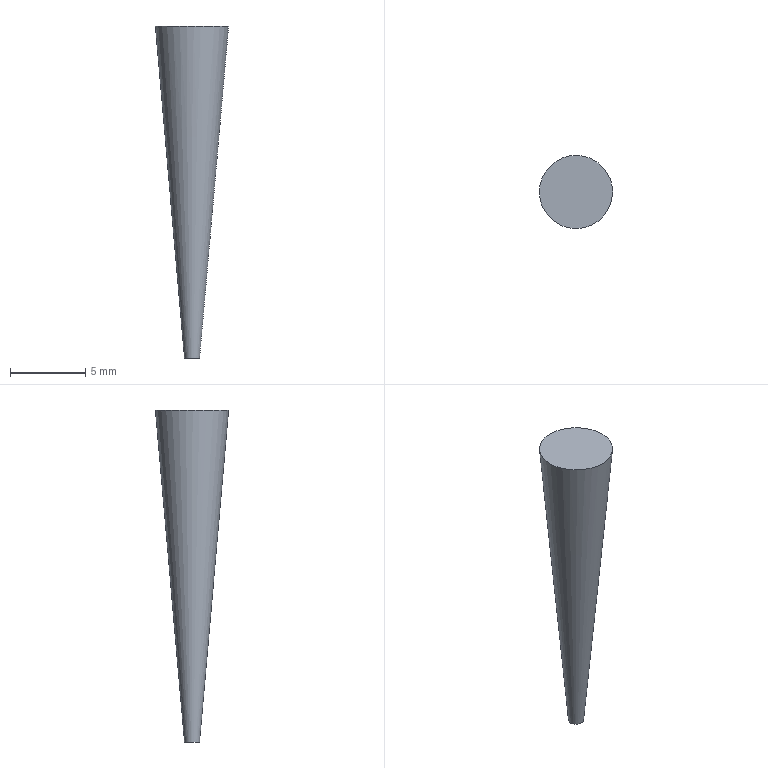Part | NX | features DATUM_CSYS 3, SKETCH 2, THRU_CURVE 1 | 1 solid | 3 faces | box 4.85 x 4.85 x 22 mm | volume 170.37 mm3 | plane 2 | spline 1